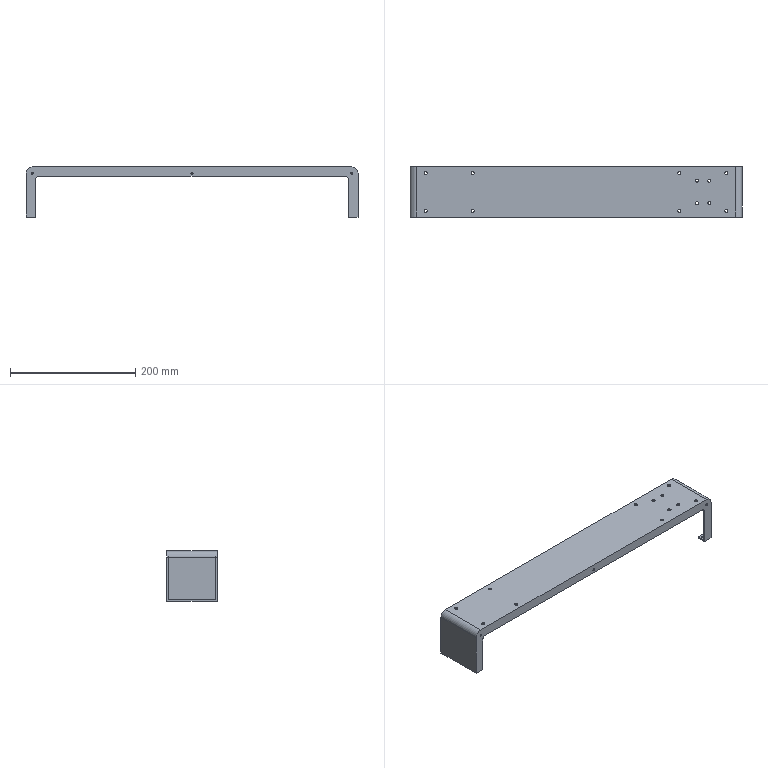Part | NX | 1 solid | 53 faces | box 530 x 80 x 80 mm | volume 138859 mm3 | cylinder 30 | plane 23 | commonest cylinder face diameters 5 x12 3.3 x7 10 x4 6 x2 16 x2 20 x2